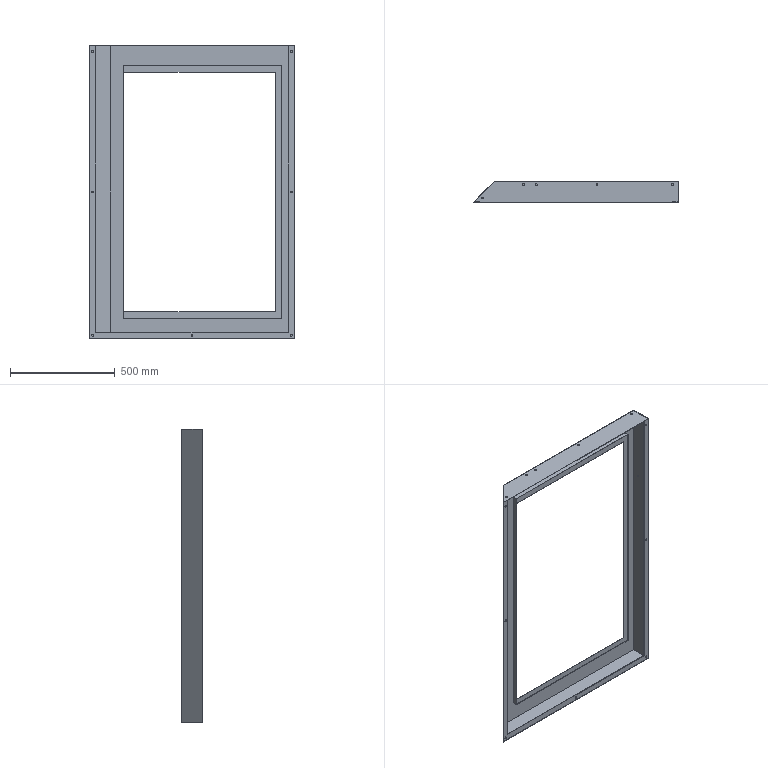Part | SolidWorks | features ICE 10, Extrusion 1 | 1 solid | 56 faces | box 980 x 100 x 1400 mm | volume 2213321 mm3 | cylinder 28 | plane 28 | commonest cylinder face diameters 9 x28